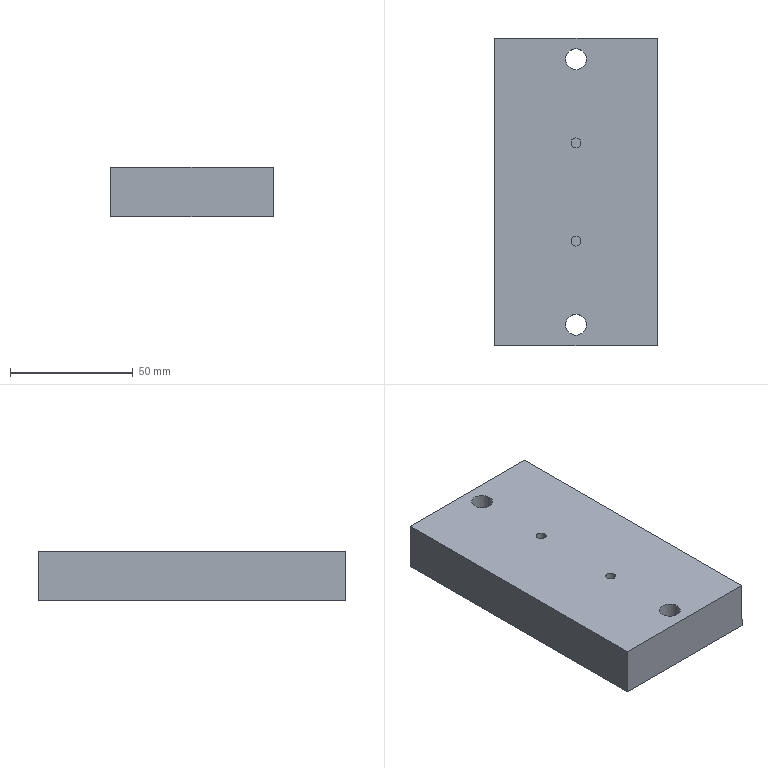CAM job | NX | 3+2 milling, drilling | part box 65.936 x 125 x 20 mm | stock box 65.936 x 125 x 20 mm
Tools:
number,name,description,diameter,corner_radius,flute_length,length,flutes
0,D63,Milling Tool-5 Parameters,63.0,0.0,50.0,75.0,2
0,D16R0波刀,Milling Tool-5 Parameters,16.0,0.0,50.0,75.0,2
0,D4R0.5,Milling Tool-5 Parameters,4.0,0.5,50.0,75.0,2
0,D6R0,Milling Tool-5 Parameters,6.0,0.0,50.0,75.0,2
0,D8R0,Milling Tool-5 Parameters,8.0,0.0,50.0,75.0,2
0,DK-D5,Countersink,5.0,0.0,0.0,60.0,2
0,D6.8钻头,Drilling Tool,6.8,0.0,35.0,50.0,2
0,D3R0,Milling Tool-5 Parameters,3.0,0.0,50.0,75.0,2
5,DK-D10,Countersink,10.0,0.0,0.0,60.0,2
27,M8,Drilling Tool,8.0,0.0,35.0,50.0,4
0,D10R0,Milling Tool-5 Parameters,10.0,0.0,50.0,75.0,2
0,D1.5R0,Milling Tool-5 Parameters,1.5,0.0,50.0,75.0,2
0,D1R0,Milling Tool-5 Parameters,1.0,0.0,50.0,75.0,2
0,D2R0,Milling Tool-5 Parameters,2.0,0.0,50.0,75.0,2
0,DJ-D3,Countersink,3.0,0.0,0.0,60.0,2
0,D2.3钻头,Drilling Tool,2.3,0.0,35.0,50.0,2
0,D1.8钻头,Drilling Tool,1.8,0.0,35.0,50.0,2
0,M2.5,Drilling Tool,2.5,0.0,35.0,50.0,4
0,M2,Drilling Tool,2.0,0.0,35.0,50.0,4
0,DJ-D8,Countersink,8.0,0.0,0.0,60.0,2
0,D12铣牙刀,Thread Mill,11.8,0.0,10.0,50.0,2
0,R1,Milling Tool-Ball Mill,2.0,1.0,20.0,20.0,2
0,D6R0EX,Milling Tool-5 Parameters,6.0,0.0,25.0,25.0,2
0,D16R0F,Milling Tool-5 Parameters,16.0,0.0,50.0,75.0,2
0,D8.5DR,Drilling Tool,8.5,0.0,35.0,50.0,2
0,D14R0,Milling Tool-5 Parameters,14.0,0.0,50.0,75.0,2
21,D2.5R0深沟,Milling Tool-5 Parameters,2.5,0.0,50.0,75.0,2
26,ZT-7.3,Drilling Tool,7.3,0.0,35.0,50.0,2
Operations:
program,operation,operation_type,tool,method,geometry_group,spindle_rpm,surface_speed,feed_per_tooth,feed_cut,feed_plunge,cut_length_mm,path_length_mm,cut_time_min,machine_time_min
A01,FACE_MILLING,FaceMilling,D63,METHOD,PN_0001,4000.0,791.0,0.15,1200.0,100.0,377.437,443.437,0.3145,0.3244
A01,FLOOR_WALL,VolumeBased25DMillingOperation,D63,METHOD,PN_0001,4000.0,791.0,0.1875,1500.0,100.0,637.218,707.171,0.4248,0.435
A01,FLOOR_WALL_COPY,VolumeBased25DMillingOperation,D63,METHOD,PN_0001,4000.0,791.0,0.15,1200.0,100.0,317.944,384.798,0.265,0.275
A02,PLANAR_MILL,PlanarMilling,D16R0波刀,METHOD,PN_0001,5500.0,276.0,0.1818,2000.0,100.0,4915.593,5055.335,2.458,2.475
A02,PLANAR_MILL_COPY,PlanarMilling,D16R0波刀,METHOD,PN_0001,5500.0,276.0,0.1818,2000.0,100.0,116.0,180.67,0.058,0.0677
A02,ZLEVEL_PROFILE,ZLevelMilling,D16R0波刀,METHOD,PN_0001,5500.0,276.0,0.3636,4000.0,100.0,1363.091,1432.797,0.3408,0.3508
A02,ZLEVEL_PROFILE_COPY_COPY_COPY,ZLevelMilling,D16R0波刀,METHOD,PN_0001,5500.0,276.0,0.3636,4000.0,100.0,1476.056,1544.786,0.369,0.3789
A02,ZLEVEL_PROFILE_COPY,ZLevelMilling,D16R0波刀,METHOD,PN_0001,5500.0,276.0,0.3636,4000.0,100.0,1136.59,1204.724,0.2841,0.294
A02,ZLEVEL_PROFILE_COPY_COPY,ZLevelMilling,D16R0波刀,METHOD,PN_0001,5500.0,276.0,0.2727,3000.0,100.0,454.262,518.855,0.1514,0.1609
A03,PLANAR_MILL_COPY_COPY,PlanarMilling,D8R0,METHOD,PN_0001,4500.0,84.0,0.1111,1000.0,100.0,204.8,384.736,0.2048,0.2288
A03,PLANAR_MILL_COPY_2,PlanarMilling,D8R0,METHOD,PN_0001,4500.0,113.0,0.0889,800.0,100.0,751.437,868.352,0.9393,0.9555
A04,FIXED_CONTOUR,SurfaceContour,D4R0.5,METHOD,PN_0001,6000.0,75.0,0.25,3000.0,100.0,5623.783,5687.119,1.875,1.884
A04,ZLEVEL_PROFILE_1,ZLevelMilling,D4R0.5,METHOD,PN_0001,6000.0,75.0,0.2083,2500.0,100.0,3985.202,4052.701,1.594,1.604
A04,ZLEVEL_PROFILE_1_COPY,ZLevelMilling,D4R0.5,METHOD,PN_0001,6000.0,75.0,0.1667,2000.0,100.0,4390.454,4455.322,2.195,2.205
A04,FIXED_CONTOUR_COPY,SurfaceContour,D4R0.5,METHOD,PN_0001,6000.0,75.0,0.2083,2500.0,100.0,4703.526,4766.281,1.881,1.891
A04,FIXED_CONTOUR_COPY_COPY,SurfaceContour,D4R0.5,METHOD,PN_0001,6000.0,75.0,0.25,3000.0,100.0,4701.245,4764.847,1.567,1.577
A05,DRILLING,Operation,DK-D10,METHOD,PN_0001,2000.0,31.0,0.05,200.0,0.0,7.4,171.882,0.037,0.0534
A05,DRILLING_COPY_1,Operation,DK-D10,METHOD,PN_0001,2000.0,31.0,0.05,200.0,0.0,11.2,179.482,0.056,0.0728
A06,DRILLING_COPY,Operation,D6.8钻头,METHOD,PN_0001,2000.0,31.0,0.05,200.0,0.0,27.0,211.082,0.135,0.1534
A07,PLANAR_MILL_1,PlanarMilling,D3R0,METHOD,PN_0001,5000.0,47.0,0.1,1000.0,100.0,498.424,685.875,0.4984,0.5231
A07,PLANAR_MILL_1_COPY,PlanarMilling,D3R0,METHOD,PN_0001,5000.0,47.0,0.02,200.0,100.0,25.677,221.178,0.1284,0.1547
A08,DRILLING_COPY_COPY,Operation,M8,METHOD,PN_0001,200.0,4.0,0.625,250.0,0.0,21.0,199.082,0.084,0.1018
B01,FACE_MILLING_COPY,FaceMilling,D63,METHOD,PN_0002,4000.0,791.0,0.25,2000.0,100.0,1132.312,1358.987,0.5662,0.5953
B01,FACE_MILLING_COPY_COPY,FaceMilling,D63,METHOD,PN_0002,4000.0,791.0,0.125,1000.0,100.0,377.437,452.437,0.3774,0.3887
B01,ZLEVEL_PROFILE_2,ZLevelMilling,D63,METHOD,PN_0002,4000.0,791.0,0.625,5000.0,100.0,2420.273,2523.476,0.4841,0.4975
B01,ZLEVEL_PROFILE_2_COPY,ZLevelMilling,D63,METHOD,PN_0002,4000.0,791.0,0.625,5000.0,100.0,2420.152,2510.91,0.484,0.4962
B01,ZLEVEL_PROFILE_2_COPY_COPY,ZLevelMilling,D63,METHOD,PN_0002,4000.0,791.0,0.5625,4500.0,100.0,2074.461,2160.717,0.461,0.4728
B01,PLANAR_MILL_1_COPY_COPY_COPY_COPY_1,PlanarMilling,D63,METHOD,PN_0002,4000.0,791.0,0.15,1200.0,100.0,167.6,227.6,0.1397,0.1487
B01,PLANAR_MILL_1_COPY_COPY_COPY,PlanarMilling,D6R0,METHOD,PN_0002,8000.0,150.0,0.125,2000.0,100.0,1313.58,1380.38,0.6568,0.6664
B01,PLANAR_MILL_1_COPY_COPY_COPY_COPY,PlanarMilling,D6R0,METHOD,PN_0002,8000.0,150.0,0.05,800.0,100.0,173.025,247.725,0.2357,0.2469
B01,CAVITY_MILL,CavityMilling,D6R0,METHOD,PN_0002,8000.0,150.0,0.2812,4500.0,100.0,2687.796,3166.688,0.5973,0.6629
B01,PLANAR_PROFILE,PlanarMilling,D6R0,METHOD,PN_0002,8000.0,150.0,0.1875,3000.0,100.0,598.8,669.6,0.1996,0.2098
B01,CAVITY_MILL_COPY_1,CavityMilling,D6R0,METHOD,PN_0002,8000.0,150.0,0.125,2000.0,100.0,240.587,302.387,0.1203,0.1296
B01,CAVITY_MILL_COPY_1_COPY_1,CavityMilling,D6R0,METHOD,PN_0002,8000.0,150.0,0.075,1200.0,100.0,241.607,303.607,0.2013,0.2106
B01,CAVITY_MILL_COPY_1_COPY_2,CavityMilling,D6R0,METHOD,PN_0002,8000.0,150.0,0.125,2000.0,100.0,241.019,302.819,0.1205,0.1298
B01,CAVITY_MILL_COPY_1_COPY_2_COPY,CavityMilling,D6R0,METHOD,PN_0002,8000.0,150.0,0.075,1200.0,100.0,241.622,303.622,0.2014,0.2107
B01,PLANAR_MILL_2_COPY_COPY,PlanarMilling,D10R0,METHOD,PN_0002,4000.0,125.0,0.125,1000.0,100.0,321.0,695.397,0.321,0.3665
B01,FACE_MILLING_1,FaceMilling,D10R0,METHOD,PN_0002,4000.0,125.0,0.1875,1500.0,100.0,1054.827,1335.16,0.7032,0.7399
B01,FACE_MILLING_1_COPY_2,FaceMilling,D10R0,METHOD,PN_0002,4000.0,125.0,0.1875,1500.0,100.0,1051.058,1330.651,0.7007,0.7373
B01,PLANAR_MILL_2_COPY_COPY_1,PlanarMilling,D10R0,METHOD,PN_0002,4000.0,125.0,0.1875,1500.0,100.0,729.155,915.21,0.4861,0.5106
B01,PLANAR_MILL_2,PlanarMilling,D10R0,METHOD,PN_0002,4000.0,125.0,0.0375,300.0,100.0,77.519,257.58,0.2584,0.2827
B01,PLANAR_MILL_2_COPY,PlanarMilling,D10R0,METHOD,PN_0002,4000.0,125.0,0.15,1200.0,100.0,345.746,639.931,0.2881,0.3215
B01,PLANAR_MILL_2_COPY_COPY_2,PlanarMilling,D10R0,METHOD,PN_0002,4000.0,125.0,0.15,1200.0,100.0,345.746,639.931,0.2881,0.3215
B01,PLANAR_MILL_2_COPY_1,PlanarMilling,D10R0,METHOD,PN_0002,4000.0,125.0,0.0375,300.0,100.0,39.544,215.04,0.1318,0.1561
B01,FACE_MILLING_1_COPY_1,FaceMilling,D10R0,METHOD,PN_0002,4000.0,125.0,0.1875,1500.0,100.0,631.761,856.738,0.4212,0.4497
B01,PLANAR_MILL_4_COPY_COPY,PlanarMilling,DJ-D8,METHOD,PN_0002,6000.0,150.0,0.05,600.0,100.0,164.591,323.474,0.2743,0.2942
B01,PLANAR_MILL_4_COPY_1,PlanarMilling,DJ-D8,METHOD,PN_0002,6000.0,150.0,0.05,600.0,100.0,164.461,323.337,0.2741,0.294
B01,DRILLING_1,Operation,DK-D5,METHOD,PN_0002,2000.0,31.0,0.0375,150.0,0.0,11.2,320.904,0.0747,0.1056
B01,DRILLING_1_COPY,Operation,DK-D5,METHOD,PN_0002,2000.0,31.0,0.0375,150.0,0.0,2.6,65.2,0.0173,0.0236
B01,DRILLING_1_COPY_2,Operation,DK-D5,METHOD,PN_0002,2000.0,31.0,0.0375,150.0,0.0,7.8,227.795,0.052,0.074
B01,DRILLING_1_COPY_2_COPY,Operation,DK-D5,METHOD,PN_0002,2000.0,31.0,0.0375,150.0,0.0,5.2,149.983,0.0347,0.0491
B01,DRILLING_1_COPY_2_COPY_COPY,Operation,DK-D5,METHOD,PN_0002,2000.0,31.0,0.0375,150.0,0.0,5.2,149.983,0.0347,0.0491
B01,DRILLING_1_COPY_1,Operation,D2.3钻头,METHOD,PN_0002,2000.0,14.0,0.025,100.0,0.0,24.4,347.304,0.244,0.2763
B01,DRILLING_1_COPY_1_COPY,Operation,D1.8钻头,METHOD,PN_0002,2000.0,14.0,0.025,100.0,0.0,7.5,75.0,0.075,0.0817
B01,DRILLING_1_COPY_1_COPY_COPY,Operation,D1.8钻头,METHOD,PN_0002,2000.0,14.0,0.025,100.0,0.0,16.5,245.195,0.165,0.1879
B01,DRILLING_1_COPY_1_COPY_COPY_COPY,Operation,D1.8钻头,METHOD,PN_0002,2000.0,14.0,0.025,100.0,0.0,12.0,163.583,0.12,0.1352
B01,DRILLING_1_COPY_1_COPY_COPY_COPY_COPY,Operation,D1.8钻头,METHOD,PN_0002,2000.0,14.0,0.025,100.0,0.0,12.0,163.583,0.12,0.1352
B01,THREAD_MILLING,ThreadMilling,D12铣牙刀,METHOD,PN_0002,4000.0,149.0,0.0375,300.0,100.0,15.937,89.435,0.0531,0.0642
B01,THREAD_MILLING_COPY,ThreadMilling,D12铣牙刀,METHOD,PN_0002,4000.0,149.0,0.0375,300.0,100.0,15.937,89.435,0.0531,0.0642
B01,DRILLING_1_COPY_1_COPY_1,Operation,M2.5,METHOD,PN_0002,400.0,3.0,0.1125,180.0,0.0,23.2,344.904,0.1289,0.1611
B01,DRILLING_1_COPY_1_COPY_1_COPY,Operation,M2,METHOD,PN_0002,400.0,2.0,0.1,160.0,0.0,7.0,74.0,0.0437,0.0504
B01,DRILLING_1_COPY_1_COPY_1_COPY_COPY,Operation,M2,METHOD,PN_0002,400.0,2.0,0.1,160.0,0.0,16.5,245.195,0.1031,0.126
B01,DRILLING_1_COPY_1_COPY_1_COPY_COPY_COPY,Operation,M2,METHOD,PN_0002,400.0,2.0,0.1,160.0,0.0,10.0,159.583,0.0625,0.0775
B01,DRILLING_1_COPY_1_COPY_1_COPY_COPY_COPY_COPY,Operation,M2,METHOD,PN_0002,400.0,2.0,0.1,160.0,0.0,10.0,159.583,0.0625,0.0775
B01,CAVITY_MILL_COPY,CavityMilling,D1.5R0,METHOD,PN_0002,8500.0,40.0,0.1176,2000.0,100.0,1820.649,3100.187,0.9103,1.077
B01,CAVITY_MILL_COPY_COPY,CavityMilling,D1.5R0,METHOD,PN_0002,8500.0,40.0,0.0706,1200.0,100.0,464.866,562.716,0.3874,0.4021
B01,PLANAR_MILL_2_COPY_COPY_COPY_COPY_COPY_COPY_1,PlanarMilling,D1.5R0,METHOD,PN_0002,8500.0,40.0,0.0353,600.0,100.0,253.337,1956.788,0.4222,0.6652
B01,PLANAR_MILL_2_COPY_COPY_COPY_COPY_COPY_COPY_1_COPY,PlanarMilling,D1.5R0,METHOD,PN_0002,8500.0,40.0,0.0588,1000.0,100.0,37.766,372.136,0.0378,0.0825
B01,PLANAR_MILL_2_COPY_COPY_COPY_COPY,PlanarMilling,D1.5R0,METHOD,PN_0002,8500.0,40.0,0.0235,400.0,100.0,327.466,398.539,0.8187,0.8291
B01,CAVITY_MILL_COPY_COPY_COPY,CavityMilling,D1.5R0,METHOD,PN_0002,8500.0,40.0,0.0353,600.0,100.0,424.896,495.896,0.7082,0.7188
B01,PLANAR_MILL_2_COPY_COPY_COPY_COPY_COPY,PlanarMilling,D1R0,METHOD,PN_0002,9000.0,28.0,0.0556,1000.0,100.0,504.615,888.3,0.5046,0.555
B01,PLANAR_MILL_3,PlanarMilling,DJ-D3,METHOD,PN_0002,6500.0,61.0,0.0615,800.0,100.0,187.298,249.298,0.2341,0.2434
B01,PLANAR_MILL_3_COPY,PlanarMilling,DJ-D3,METHOD,PN_0002,6500.0,61.0,0.0615,800.0,100.0,78.536,151.536,0.0982,0.1091
B01,PLANAR_MILL_3_COPY_1,PlanarMilling,DJ-D3,METHOD,PN_0002,6500.0,61.0,0.0615,800.0,100.0,47.632,199.368,0.0595,0.0809
B01,PLANAR_MILL_3_COPY_1_COPY,PlanarMilling,DJ-D3,METHOD,PN_0002,6500.0,61.0,0.0615,800.0,100.0,95.336,266.194,0.1192,0.1425
B01,PLANAR_MILL_3_COPY_1_COPY_COPY,PlanarMilling,DJ-D3,METHOD,PN_0002,6500.0,61.0,0.0615,800.0,100.0,99.0,161.0,0.1238,0.1331
B01,PLANAR_MILL_3_COPY_1_COPY_COPY_COPY_1,PlanarMilling,DJ-D3,METHOD,PN_0002,6500.0,61.0,0.0615,800.0,100.0,105.0,167.0,0.1313,0.1406
B01,PLANAR_MILL_3_COPY_1_COPY_COPY_COPY,PlanarMilling,DJ-D3,METHOD,PN_0002,6500.0,61.0,0.0615,800.0,100.0,164.711,226.711,0.2059,0.2152
B01,PLANAR_MILL_3_COPY_1_COPY_COPY_COPY_COPY,PlanarMilling,DJ-D3,METHOD,PN_0002,6500.0,61.0,0.0615,800.0,100.0,105.522,167.522,0.1319,0.1412
B01,PLANAR_MILL_3_COPY_1_COPY_COPY_COPY_COPY_COPY,PlanarMilling,DJ-D3,METHOD,PN_0002,6500.0,61.0,0.0615,800.0,100.0,87.317,148.917,0.1091,0.1184
B01,PLANAR_MILL_3_COPY_1_COPY_COPY_COPY_COPY_COPY_COPY,PlanarMilling,DJ-D3,METHOD,PN_0002,6500.0,61.0,0.0615,800.0,100.0,78.425,140.025,0.098,0.1073
B01,PLANAR_MILL_3_COPY_1_COPY_COPY_COPY_COPY_COPY_COPY_1,PlanarMilling,DJ-D3,METHOD,PN_0002,6500.0,61.0,0.0615,800.0,100.0,87.317,148.917,0.1091,0.1184
B01,PLANAR_MILL_3_COPY_1_COPY_COPY_COPY_COPY_COPY_COPY_1_COPY,PlanarMilling,DJ-D3,METHOD,PN_0002,6500.0,61.0,0.0615,800.0,100.0,78.425,140.025,0.098,0.1073
C01,CAVITY_MILL_1,CavityMilling,D6R0EX,METHOD,PN_0001,8500.0,160.0,0.1765,3000.0,100.0,10987.552,11417.366,3.663,3.71
C01,PLANAR_MILL_5,PlanarMilling,D6R0EX,METHOD,PN_0001,8000.0,150.0,0.125,2000.0,100.0,612.645,1130.754,0.3063,0.3612
C01,PLANAR_MILL_5_COPY,PlanarMilling,D6R0EX,METHOD,PN_0001,8000.0,150.0,0.0375,600.0,100.0,87.992,154.992,0.1467,0.1567
C01,ZLEVEL_PROFILE_3_COPY_1,ZLevelMilling,D6R0EX,METHOD,PN_0001,8000.0,150.0,0.0375,600.0,100.0,315.792,1023.263,0.5263,0.6179
C01,PLANAR_MILL_5_COPY_1_COPY_COPY_COPY_COPY_COPY,PlanarMilling,D6R0EX,METHOD,PN_0001,8000.0,150.0,0.025,400.0,100.0,9.043,71.043,0.0226,0.0319
C01,PLANAR_MILL_5_COPY_1_COPY_COPY_COPY_COPY_COPY_COPY,PlanarMilling,D6R0EX,METHOD,PN_0001,8000.0,150.0,0.025,400.0,100.0,9.043,71.043,0.0226,0.0319
C01,PLANAR_MILL_5_COPY_1,PlanarMilling,D10R0,METHOD,PN_0001,6000.0,113.0,0.0833,1000.0,100.0,104.0,172.368,0.104,0.1143
C01,PLANAR_MILL_5_COPY_1_COPY,PlanarMilling,D10R0,METHOD,PN_0001,6000.0,113.0,0.0833,1000.0,100.0,106.0,166.0,0.106,0.115
C01,PLANAR_MILL_5_COPY_1_COPY_COPY,PlanarMilling,D10R0,METHOD,PN_0001,6000.0,113.0,0.0833,1000.0,100.0,106.0,166.0,0.106,0.115
C01,PLANAR_MILL_5_COPY_1_COPY_COPY_COPY,PlanarMilling,D10R0,METHOD,PN_0001,6000.0,113.0,0.0833,1000.0,100.0,106.0,166.0,0.106,0.115
C01,PLANAR_MILL_5_COPY_1_COPY_COPY_COPY_COPY,PlanarMilling,D10R0,METHOD,PN_0001,6000.0,113.0,0.0833,1000.0,100.0,106.0,173.924,0.106,0.1162
C01,PLANAR_MILL_5_COPY_1_COPY_COPY_COPY_COPY_COPY_COPY_COPY_COPY,PlanarMilling,D10R0,METHOD,PN_0001,6000.0,188.0,0.1,1200.0,100.0,664.028,724.028,0.5534,0.5624
C01,PLANAR_MILL_5_COPY_1_COPY_COPY_COPY_COPY_COPY_COPY_COPY_COPY_COPY,PlanarMilling,D10R0,METHOD,PN_0001,6000.0,188.0,0.1,1200.0,100.0,390.859,450.859,0.3257,0.3347
C01,PLANAR_MILL_5_COPY_1_COPY_COPY_COPY_COPY_COPY_COPY_COPY_COPY_COPY_1,PlanarMilling,D10R0,METHOD,PN_0001,6000.0,188.0,0.0667,800.0,100.0,664.028,724.028,0.83,0.839
C01,PLANAR_MILL_5_COPY_1_COPY_COPY_COPY_COPY_COPY_COPY_COPY_COPY_COPY_COPY,PlanarMilling,D10R0,METHOD,PN_0001,6000.0,188.0,0.0667,800.0,100.0,390.859,450.899,0.4886,0.4976
C01,CAVITY_MILL_1_COPY,CavityMilling,D2.5R0深沟,METHOD,PN_0001,6000.0,37.0,0.125,1500.0,100.0,3557.785,5066.589,2.372,2.556
C01,PROFILE_3D,PlanarMilling,D2.5R0深沟,METHOD,PN_0001,6000.0,47.0,0.0167,200.0,100.0,65.185,104.785,0.3259,0.3299
C01,PROFILE_3D_COPY,PlanarMilling,D2.5R0深沟,METHOD,PN_0001,6000.0,47.0,0.0167,200.0,100.0,65.185,104.785,0.3259,0.3299
C01,FIXED_CONTOUR_3,SurfaceContour,R1,METHOD,PN_0001,8000.0,50.0,0.0938,1500.0,100.0,3343.476,3772.557,2.229,2.289
C01,FIXED_CONTOUR_3_COPY,SurfaceContour,R1,METHOD,PN_0001,8000.0,50.0,0.0938,1500.0,100.0,1796.359,2104.916,1.198,1.243
C01,PLANAR_MILL_3_COPY_1_COPY_COPY_COPY_COPY_COPY_COPY_1_COPY_COPY,PlanarMilling,DJ-D3,METHOD,PN_0001,5500.0,51.0,0.0909,1000.0,100.0,200.7,262.7,0.2007,0.21
C01,PLANAR_MILL_3_COPY_1_COPY_COPY_COPY_COPY_COPY_COPY_1_COPY_COPY_COPY,PlanarMilling,DJ-D3,METHOD,PN_0001,5500.0,51.0,0.0909,1000.0,100.0,108.0,310.0,0.108,0.1344
C01,PLANAR_MILL_7,PlanarMilling,DK-D5,METHOD,PN_0001,4500.0,70.0,0.0667,600.0,100.0,102.816,399.616,0.1714,0.201
工装1-1,FACE_MILLING_COPY_1,FaceMilling,D63,METHOD,工装1-1,4000.0,791.0,0.15,1200.0,100.0,437.879,503.879,0.3649,0.3748
工装1-1,PLANAR_MILL_COPY_1,PlanarMilling,D16R0波刀,METHOD,工装1-1,5500.0,276.0,0.1818,2000.0,100.0,7805.846,8034.883,3.903,3.929
工装1-1,PLANAR_MILL_COPY_COPY_COPY_COPY,PlanarMilling,D16R0F,METHOD,工装1-1,4500.0,84.0,0.0889,800.0,100.0,452.267,595.067,0.5653,0.5868
工装1-1,DRILLING_COPY_2,Operation,DK-D10,METHOD,工装1-1,2000.0,31.0,0.05,200.0,0.0,23.2,340.688,0.116,0.1477
工装1-1,DRILLING_COPY_2_COPY,Operation,DK-D10,METHOD,工装1-1,2000.0,31.0,0.05,200.0,0.0,14.0,301.693,0.07,0.0988
工装1-1,DRILLING_COPY_2_COPY_1,Operation,D8.5DR,METHOD,工装1-1,2000.0,53.0,0.05,200.0,0.0,43.0,288.089,0.215,0.2395
工装1-1,DRILLING_COPY_2_COPY_1_COPY,Operation,D8.5DR,METHOD,工装1-1,2000.0,53.0,0.0375,150.0,0.0,93.0,343.082,0.62,0.645
工装1-1,DRILLING_COPY_2_COPY_1_COPY_COPY,Operation,D14R0,METHOD,工装1-1,800.0,35.0,0.0625,100.0,0.0,49.0,255.082,0.49,0.5106
工装1-1,PLANAR_MILL_COPY_1_COPY,PlanarMilling,D2R0,METHOD,工装1-1,6500.0,40.0,0.0923,1200.0,100.0,1239.111,1582.306,1.033,1.079
工装1-1,PLANAR_MILL_COPY_1_COPY_COPY,PlanarMilling,D2R0,METHOD,工装1-1,6500.0,40.0,0.0154,200.0,100.0,34.0,398.767,0.17,0.2205
工装1-1,PLANAR_MILL_COPY_COPY_COPY_COPY_COPY,PlanarMilling,DK-D10,METHOD,工装1-1,4000.0,125.0,0.15,1200.0,100.0,404.87,467.87,0.3374,0.3468
工装1-1,PLANAR_MILL_COPY_COPY_COPY_COPY_COPY_COPY,PlanarMilling,DK-D10,METHOD,工装1-1,4000.0,125.0,0.15,1200.0,100.0,89.115,275.123,0.0743,0.0992
工装1-2,FACE_MILLING_COPY_1_COPY,FaceMilling,D63,METHOD,工装1-2,4000.0,791.0,0.1875,1500.0,100.0,1751.515,2024.951,1.168,1.202
工装1-2,FACE_MILLING_COPY_1_COPY_COPY,FaceMilling,D63,METHOD,工装1-2,4000.0,791.0,0.125,1000.0,100.0,437.879,507.879,0.4379,0.4484
工装1-2,FLOOR_WALL_1,VolumeBased25DMillingOperation,D16R0波刀,METHOD,工装1-2,5500.0,276.0,0.1818,2000.0,100.0,4824.863,5431.262,2.412,2.479
工装1-2,CAVITY_MILL_2,CavityMilling,D16R0波刀,METHOD,工装1-2,5000.0,251.0,0.2,2000.0,100.0,993.489,1057.289,0.4967,0.5063
工装1-2,FLOOR_WALL_1_COPY,VolumeBased25DMillingOperation,D16R0F,METHOD,工装1-2,4000.0,201.0,0.1,800.0,100.0,371.743,741.418,0.4647,0.5128
工装1-2,DRILLING_COPY_2_COPY_1_COPY_COPY_COPY,Operation,D14R0,METHOD,工装1-2,800.0,35.0,0.0625,100.0,0.0,19.0,315.013,0.19,0.2196
工装1-3,CAVITY_MILL_2_COPY,CavityMilling,D8R0,METHOD,工装1-2,4974.0,125.0,0.1005,1000.0,100.0,1632.809,1696.809,1.633,1.642
工装1-3,PLANAR_MILL_6,PlanarMilling,D8R0,METHOD,工装1-2,4000.0,100.0,0.0375,300.0,100.0,176.388,365.6,0.6578,0.6831
工装1-3,PLANAR_MILL_COPY_COPY_COPY_COPY_COPY_COPY_COPY,PlanarMilling,DK-D10,METHOD,工装1-2,4000.0,125.0,0.15,1200.0,100.0,323.872,386.872,0.2699,0.2793
工装1-3,PLANAR_MILL_COPY_COPY_COPY_COPY_COPY_COPY_COPY_COPY,PlanarMilling,DK-D10,METHOD,工装1-2,4000.0,125.0,0.15,1200.0,100.0,45.699,175.699,0.0381,0.0546
工装2-1,FACE_MILLING_COPY_1_COPY_1,FaceMilling,D63,METHOD,工装2-1,4000.0,791.0,0.15,1200.0,100.0,367.052,433.052,0.3059,0.3158
工装2-1,PLANAR_MILL_COPY_1_COPY_1,PlanarMilling,D16R0波刀,METHOD,工装2-1,5500.0,276.0,0.1818,2000.0,100.0,6307.364,6527.335,3.154,3.179
工装2-1,CAVITY_MILL_3,CavityMilling,D16R0波刀,METHOD,工装2-1,5500.0,276.0,0.1818,2000.0,100.0,3688,3817.149,1.844,1.862
工装2-1,PLANAR_MILL_COPY_1_COPY_1_COPY,PlanarMilling,D16R0F,METHOD,工装2-1,5500.0,276.0,0.0727,800.0,100.0,1176.331,1321.046,1.47,1.489
工装2-1,CAVITY_MILL_3_COPY,CavityMilling,D4R0.5,METHOD,工装2-1,5500.0,276.0,0.1818,2000.0,100.0,10070.901,10276.819,5.035,5.062
工装2-1,FIXED_CONTOUR_2,SurfaceContour,D4R0.5,METHOD,工装2-1,6000.0,75.0,0.25,3000.0,100.0,17919.714,17991.791,5.973,5.984
工装2-1,FIXED_CONTOUR_2_COPY,SurfaceContour,D4R0.5,METHOD,工装2-1,6000.0,75.0,0.25,3000.0,100.0,13455.043,13526.038,4.485,4.495
A,DRILLING_2,Operation,DK-D10,METHOD,工装2-22,2000.0,62.0,0.03,120.0,0.0,12.2,202.862,0.1017,0.1207
A,DRILLING_2_COPY,Operation,DK-D10,METHOD,工装2-22,2000.0,62.0,0.03,120.0,0.0,8.2,127.631,0.0683,0.0803
B,DRILLING_2_COPY_1,Operation,ZT-7.3,METHOD,工装2-22,2000.0,62.0,0.03,120.0,0.0,64.0,306.462,0.5333,0.5576
C,DRILLING_2_COPY_1_COPY,Operation,M8,METHOD,工装2-22,400.0,10.0,0.3125,500.0,0.0,34.0,246.462,0.068,0.0892
D,PLANAR_MILL_4,PlanarMilling,D2.5R0深沟,METHOD,工装2-22,4000.0,31.0,0.025,200.0,100.0,812.406,989.754,4.062,4.08
D,PLANAR_MILL_4_COPY_2,PlanarMilling,D2.5R0深沟,METHOD,工装2-22,4000.0,31.0,0.025,200.0,100.0,33.991,406.317,0.17,0.2072